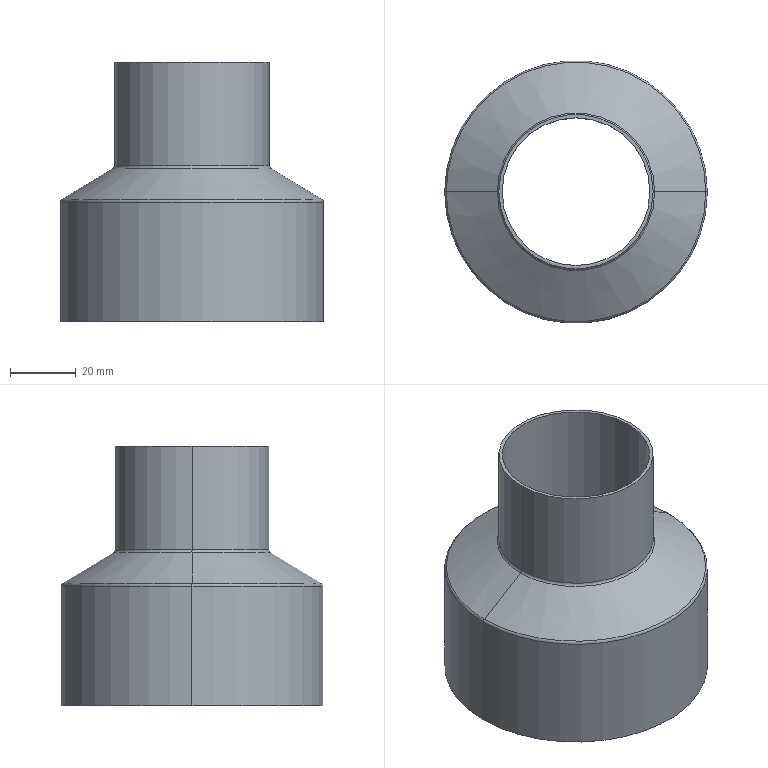Part | SolidWorks | features 3DProfileFeature 2, ICE 2, Blend 1, Fillet 1, Shell 1 | 1 solid | 18 faces | box 80 x 80 x 79 mm | volume 17561 mm3 | cylinder 8 | torus 4 | cone 4 | plane 2 | commonest cylinder face diameters 45 x2 47 x2 78 x2 80 x2
STEP:
#1=CARTESIAN_POINT('',(-23.5,0.,10.563));
#2=VERTEX_POINT('',#1);
#3=CARTESIAN_POINT('',(23.5,0.,10.563));
#4=VERTEX_POINT('',#3);
#5=CARTESIAN_POINT('',(0.,0.,10.563));
#6=DIRECTION('',(0.,0.,1.));
#7=DIRECTION('',(1.,0.,0.));
#8=AXIS2_PLACEMENT_3D('',#5,#6,#7);
#9=CIRCLE('',#8,23.5);
#10=EDGE_CURVE('',#2,#4,#9,.T.);
#11=ORIENTED_EDGE('',*,*,#10,.F.);
#12=CARTESIAN_POINT('',(-23.982,0.,9.708));
#13=VERTEX_POINT('',#12);
#14=CARTESIAN_POINT('',(-24.5,0.,10.563));
#15=DIRECTION('',(0.,1.,0.));
#16=DIRECTION('',(-1.,0.,0.));
#17=AXIS2_PLACEMENT_3D('',#14,#15,#16);
#18=CIRCLE('',#17,1.);
#19=EDGE_CURVE('',#2,#13,#18,.T.);
#20=ORIENTED_EDGE('',*,*,#19,.T.);
#21=CARTESIAN_POINT('',(23.982,0.,9.708));
#22=VERTEX_POINT('',#21);
#23=CARTESIAN_POINT('',(0.,0.,9.708));
#24=DIRECTION('',(0.,0.,-1.));
#25=DIRECTION('',(1.,0.,0.));
#26=AXIS2_PLACEMENT_3D('',#23,#24,#25);
#27=CIRCLE('',#26,23.982);
#28=EDGE_CURVE('',#22,#13,#27,.T.);
#29=ORIENTED_EDGE('',*,*,#28,.F.);
#30=CARTESIAN_POINT('',(24.5,0.,10.563));
#31=DIRECTION('',(0.,-1.,0.));
#32=DIRECTION('',(0.,0.,-1.));
#33=AXIS2_PLACEMENT_3D('',#30,#31,#32);
#34=CIRCLE('',#33,1.);
#35=EDGE_CURVE('',#4,#22,#34,.T.);
#36=ORIENTED_EDGE('',*,*,#35,.F.);
#37=EDGE_LOOP('',(#11,#20,#29,#36));
#38=FACE_OUTER_BOUND('',#37,.T.);
#39=CARTESIAN_POINT('',(0.,0.,10.563));
#40=DIRECTION('',(0.,0.,1.));
#41=DIRECTION('',(1.,0.,0.));
#42=AXIS2_PLACEMENT_3D('',#39,#40,#41);
#43=TOROIDAL_SURFACE('',#42,24.5,1.);
#44=ADVANCED_FACE('',(#38),#43,.F.);
#45=CARTESIAN_POINT('',(-40.,0.,-0.5633));
#46=VERTEX_POINT('',#45);
#47=CARTESIAN_POINT('',(40.,0.,-0.5633));
#48=VERTEX_POINT('',#47);
#49=CARTESIAN_POINT('',(0.,0.,-0.5633));
#50=DIRECTION('',(0.,0.,-1.));
#51=DIRECTION('',(1.,0.,0.));
#52=AXIS2_PLACEMENT_3D('',#49,#50,#51);
#53=CIRCLE('',#52,40.);
#54=EDGE_CURVE('',#46,#48,#53,.T.);
#55=ORIENTED_EDGE('',*,*,#54,.F.);
#56=CARTESIAN_POINT('',(-39.518,0.,0.2919));
#57=VERTEX_POINT('',#56);
#58=CARTESIAN_POINT('',(-39.,0.,-0.5633));
#59=DIRECTION('',(0.,1.,0.));
#60=DIRECTION('',(-1.,0.,0.));
#61=AXIS2_PLACEMENT_3D('',#58,#59,#60);
#62=CIRCLE('',#61,1.);
#63=EDGE_CURVE('',#46,#57,#62,.T.);
#64=ORIENTED_EDGE('',*,*,#63,.T.);
#65=CARTESIAN_POINT('',(39.518,0.,0.2919));
#66=VERTEX_POINT('',#65);
#67=CARTESIAN_POINT('',(0.,0.,0.2919));
#68=DIRECTION('',(0.,0.,1.));
#69=DIRECTION('',(-1.,0.,0.));
#70=AXIS2_PLACEMENT_3D('',#67,#68,#69);
#71=CIRCLE('',#70,39.518);
#72=EDGE_CURVE('',#66,#57,#71,.T.);
#73=ORIENTED_EDGE('',*,*,#72,.F.);
#74=CARTESIAN_POINT('',(39.,0.,-0.5633));
#75=DIRECTION('',(0.,-1.,0.));
#76=DIRECTION('',(0.,0.,-1.));
#77=AXIS2_PLACEMENT_3D('',#74,#75,#76);
#78=CIRCLE('',#77,1.);
#79=EDGE_CURVE('',#48,#66,#78,.T.);
#80=ORIENTED_EDGE('',*,*,#79,.F.);
#81=EDGE_LOOP('',(#55,#64,#73,#80));
#82=FACE_OUTER_BOUND('',#81,.T.);
#83=CARTESIAN_POINT('',(0.,0.,-0.5633));
#84=DIRECTION('',(0.,0.,1.));
#85=DIRECTION('',(1.,0.,0.));
#86=AXIS2_PLACEMENT_3D('',#83,#84,#85);
#87=TOROIDAL_SURFACE('',#86,39.,1.);
#88=ADVANCED_FACE('',(#82),#87,.T.);
#89=CARTESIAN_POINT('',(-22.5,0.,42.));
#90=VERTEX_POINT('',#89);
#91=CARTESIAN_POINT('',(22.5,0.,42.));
#92=VERTEX_POINT('',#91);
#93=CARTESIAN_POINT('',(0.,0.,42.));
#94=DIRECTION('',(0.,0.,1.));
#95=DIRECTION('',(1.,0.,0.));
#96=AXIS2_PLACEMENT_3D('',#93,#94,#95);
#97=CIRCLE('',#96,22.5);
#98=EDGE_CURVE('',#90,#92,#97,.T.);
#99=ORIENTED_EDGE('',*,*,#98,.T.);
#100=CARTESIAN_POINT('',(22.5,0.,9.437));
#101=VERTEX_POINT('',#100);
#102=CARTESIAN_POINT('',(22.5,0.,42.));
#103=DIRECTION('',(0.,0.,-1.));
#104=VECTOR('',#103,1000.);
#105=LINE('',#102,#104);
#106=EDGE_CURVE('',#92,#101,#105,.T.);
#107=ORIENTED_EDGE('',*,*,#106,.T.);
#108=CARTESIAN_POINT('',(-22.5,0.,9.437));
#109=VERTEX_POINT('',#108);
#110=CARTESIAN_POINT('',(0.,0.,9.437));
#111=DIRECTION('',(0.,0.,1.));
#112=DIRECTION('',(-1.,0.,0.));
#113=AXIS2_PLACEMENT_3D('',#110,#111,#112);
#114=CIRCLE('',#113,22.5);
#115=EDGE_CURVE('',#109,#101,#114,.T.);
#116=ORIENTED_EDGE('',*,*,#115,.F.);
#117=CARTESIAN_POINT('',(-22.5,0.,42.));
#118=DIRECTION('',(0.,0.,-1.));
#119=VECTOR('',#118,1000.);
#120=LINE('',#117,#119);
#121=EDGE_CURVE('',#90,#109,#120,.T.);
#122=ORIENTED_EDGE('',*,*,#121,.F.);
#123=EDGE_LOOP('',(#99,#107,#116,#122));
#124=FACE_OUTER_BOUND('',#123,.T.);
#125=CARTESIAN_POINT('',(0.,0.,42.));
#126=DIRECTION('',(0.,0.,-1.));
#127=DIRECTION('',(-1.,0.,0.));
#128=AXIS2_PLACEMENT_3D('',#125,#126,#127);
#129=CYLINDRICAL_SURFACE('',#128,22.5);
#130=ADVANCED_FACE('',(#124),#129,.F.);
#131=CARTESIAN_POINT('',(39.,0.,-37.));
#132=VERTEX_POINT('',#131);
#133=CARTESIAN_POINT('',(-39.,0.,-37.));
#134=VERTEX_POINT('',#133);
#135=CARTESIAN_POINT('',(0.,0.,-37.));
#136=DIRECTION('',(0.,0.,-1.));
#137=DIRECTION('',(-1.,0.,0.));
#138=AXIS2_PLACEMENT_3D('',#135,#136,#137);
#139=CIRCLE('',#138,39.);
#140=EDGE_CURVE('',#132,#134,#139,.T.);
#141=ORIENTED_EDGE('',*,*,#140,.T.);
#142=CARTESIAN_POINT('',(-39.,0.,-0.5633));
#143=VERTEX_POINT('',#142);
#144=CARTESIAN_POINT('',(-39.,0.,-37.));
#145=DIRECTION('',(0.,0.,1.));
#146=VECTOR('',#145,1000.);
#147=LINE('',#144,#146);
#148=EDGE_CURVE('',#134,#143,#147,.T.);
#149=ORIENTED_EDGE('',*,*,#148,.T.);
#150=CARTESIAN_POINT('',(39.,0.,-0.5633));
#151=VERTEX_POINT('',#150);
#152=CARTESIAN_POINT('',(0.,0.,-0.5633));
#153=DIRECTION('',(0.,0.,-1.));
#154=DIRECTION('',(-1.,0.,0.));
#155=AXIS2_PLACEMENT_3D('',#152,#153,#154);
#156=CIRCLE('',#155,39.);
#157=EDGE_CURVE('',#151,#143,#156,.T.);
#158=ORIENTED_EDGE('',*,*,#157,.F.);
#159=CARTESIAN_POINT('',(39.,0.,-37.));
#160=DIRECTION('',(0.,0.,1.));
#161=VECTOR('',#160,1000.);
#162=LINE('',#159,#161);
#163=EDGE_CURVE('',#132,#151,#162,.T.);
#164=ORIENTED_EDGE('',*,*,#163,.F.);
#165=EDGE_LOOP('',(#141,#149,#158,#164));
#166=FACE_OUTER_BOUND('',#165,.T.);
#167=CARTESIAN_POINT('',(0.,0.,-37.));
#168=DIRECTION('',(0.,0.,1.));
#169=DIRECTION('',(1.,0.,0.));
#170=AXIS2_PLACEMENT_3D('',#167,#168,#169);
#171=CYLINDRICAL_SURFACE('',#170,39.);
#172=ADVANCED_FACE('',(#166),#171,.F.);
#173=ORIENTED_EDGE('',*,*,#115,.T.);
#174=CARTESIAN_POINT('',(22.982,0.,9.145));
#175=DIRECTION('',(0.8552,0.,-0.5183));
#176=VECTOR('',#175,1000.);
#177=LINE('',#174,#176);
#178=EDGE_CURVE('',#101,#151,#177,.T.);
#179=ORIENTED_EDGE('',*,*,#178,.T.);
#180=ORIENTED_EDGE('',*,*,#157,.T.);
#181=CARTESIAN_POINT('',(-22.982,0.,9.145));
#182=DIRECTION('',(-0.8552,0.,-0.5183));
#183=VECTOR('',#182,1000.);
#184=LINE('',#181,#183);
#185=EDGE_CURVE('',#109,#143,#184,.T.);
#186=ORIENTED_EDGE('',*,*,#185,.F.);
#187=EDGE_LOOP('',(#173,#179,#180,#186));
#188=FACE_OUTER_BOUND('',#187,.T.);
#189=CARTESIAN_POINT('',(0.,0.,9.145));
#190=DIRECTION('',(0.,0.,-1.));
#191=DIRECTION('',(-1.,0.,0.));
#192=AXIS2_PLACEMENT_3D('',#189,#190,#191);
#193=CONICAL_SURFACE('',#192,22.982,1.026);
#194=ADVANCED_FACE('',(#188),#193,.F.);
#195=CARTESIAN_POINT('',(23.5,0.,42.));
#196=VERTEX_POINT('',#195);
#197=CARTESIAN_POINT('',(-23.5,0.,42.));
#198=VERTEX_POINT('',#197);
#199=CARTESIAN_POINT('',(0.,0.,42.));
#200=DIRECTION('',(0.,0.,1.));
#201=DIRECTION('',(1.,0.,0.));
#202=AXIS2_PLACEMENT_3D('',#199,#200,#201);
#203=CIRCLE('',#202,23.5);
#204=EDGE_CURVE('',#196,#198,#203,.T.);
#205=ORIENTED_EDGE('',*,*,#204,.F.);
#206=CARTESIAN_POINT('',(23.5,0.,42.));
#207=DIRECTION('',(0.,0.,-1.));
#208=VECTOR('',#207,1000.);
#209=LINE('',#206,#208);
#210=EDGE_CURVE('',#196,#4,#209,.T.);
#211=ORIENTED_EDGE('',*,*,#210,.T.);
#212=CARTESIAN_POINT('',(0.,0.,10.563));
#213=DIRECTION('',(0.,0.,1.));
#214=DIRECTION('',(1.,0.,0.));
#215=AXIS2_PLACEMENT_3D('',#212,#213,#214);
#216=CIRCLE('',#215,23.5);
#217=EDGE_CURVE('',#4,#2,#216,.T.);
#218=ORIENTED_EDGE('',*,*,#217,.T.);
#219=CARTESIAN_POINT('',(-23.5,0.,42.));
#220=DIRECTION('',(0.,0.,-1.));
#221=VECTOR('',#220,1000.);
#222=LINE('',#219,#221);
#223=EDGE_CURVE('',#198,#2,#222,.T.);
#224=ORIENTED_EDGE('',*,*,#223,.F.);
#225=EDGE_LOOP('',(#205,#211,#218,#224));
#226=FACE_OUTER_BOUND('',#225,.T.);
#227=CARTESIAN_POINT('',(0.,0.,42.));
#228=DIRECTION('',(0.,0.,-1.));
#229=DIRECTION('',(-1.,0.,0.));
#230=AXIS2_PLACEMENT_3D('',#227,#228,#229);
#231=CYLINDRICAL_SURFACE('',#230,23.5);
#232=ADVANCED_FACE('',(#226),#231,.T.);
#233=CARTESIAN_POINT('',(-40.,0.,-37.));
#234=VERTEX_POINT('',#233);
#235=CARTESIAN_POINT('',(40.,0.,-37.));
#236=VERTEX_POINT('',#235);
#237=CARTESIAN_POINT('',(0.,0.,-37.));
#238=DIRECTION('',(0.,0.,-1.));
#239=DIRECTION('',(-1.,0.,0.));
#240=AXIS2_PLACEMENT_3D('',#237,#238,#239);
#241=CIRCLE('',#240,40.);
#242=EDGE_CURVE('',#234,#236,#241,.T.);
#243=ORIENTED_EDGE('',*,*,#242,.F.);
#244=CARTESIAN_POINT('',(-40.,0.,-37.));
#245=DIRECTION('',(0.,0.,1.));
#246=VECTOR('',#245,1000.);
#247=LINE('',#244,#246);
#248=EDGE_CURVE('',#234,#46,#247,.T.);
#249=ORIENTED_EDGE('',*,*,#248,.T.);
#250=ORIENTED_EDGE('',*,*,#54,.T.);
#251=CARTESIAN_POINT('',(40.,0.,-37.));
#252=DIRECTION('',(0.,0.,1.));
#253=VECTOR('',#252,1000.);
#254=LINE('',#251,#253);
#255=EDGE_CURVE('',#236,#48,#254,.T.);
#256=ORIENTED_EDGE('',*,*,#255,.F.);
#257=EDGE_LOOP('',(#243,#249,#250,#256));
#258=FACE_OUTER_BOUND('',#257,.T.);
#259=CARTESIAN_POINT('',(0.,0.,-37.));
#260=DIRECTION('',(0.,0.,1.));
#261=DIRECTION('',(1.,0.,0.));
#262=AXIS2_PLACEMENT_3D('',#259,#260,#261);
#263=CYLINDRICAL_SURFACE('',#262,40.);
#264=ADVANCED_FACE('',(#258),#263,.T.);
#265=CARTESIAN_POINT('',(0.,0.,9.708));
#266=DIRECTION('',(0.,0.,-1.));
#267=DIRECTION('',(1.,0.,0.));
#268=AXIS2_PLACEMENT_3D('',#265,#266,#267);
#269=CIRCLE('',#268,23.982);
#270=EDGE_CURVE('',#13,#22,#269,.T.);
#271=ORIENTED_EDGE('',*,*,#270,.T.);
#272=CARTESIAN_POINT('',(23.5,0.,10.));
#273=DIRECTION('',(0.8552,0.,-0.5183));
#274=VECTOR('',#273,1000.);
#275=LINE('',#272,#274);
#276=EDGE_CURVE('',#22,#66,#275,.T.);
#277=ORIENTED_EDGE('',*,*,#276,.T.);
#278=ORIENTED_EDGE('',*,*,#72,.T.);
#279=CARTESIAN_POINT('',(-23.5,0.,10.));
#280=DIRECTION('',(-0.8552,0.,-0.5183));
#281=VECTOR('',#280,1000.);
#282=LINE('',#279,#281);
#283=EDGE_CURVE('',#13,#57,#282,.T.);
#284=ORIENTED_EDGE('',*,*,#283,.F.);
#285=EDGE_LOOP('',(#271,#277,#278,#284));
#286=FACE_OUTER_BOUND('',#285,.T.);
#287=CARTESIAN_POINT('',(0.,0.,10.));
#288=DIRECTION('',(0.,0.,-1.));
#289=DIRECTION('',(-1.,0.,0.));
#290=AXIS2_PLACEMENT_3D('',#287,#288,#289);
#291=CONICAL_SURFACE('',#290,23.5,1.026);
#292=ADVANCED_FACE('',(#286),#291,.T.);
#293=ORIENTED_EDGE('',*,*,#276,.F.);
#294=ORIENTED_EDGE('',*,*,#28,.T.);
#295=ORIENTED_EDGE('',*,*,#283,.T.);
#296=CARTESIAN_POINT('',(0.,0.,0.2919));
#297=DIRECTION('',(0.,0.,1.));
#298=DIRECTION('',(-1.,0.,0.));
#299=AXIS2_PLACEMENT_3D('',#296,#297,#298);
#300=CIRCLE('',#299,39.518);
#301=EDGE_CURVE('',#57,#66,#300,.T.);
#302=ORIENTED_EDGE('',*,*,#301,.T.);
#303=EDGE_LOOP('',(#293,#294,#295,#302));
#304=FACE_OUTER_BOUND('',#303,.T.);
#305=CARTESIAN_POINT('',(0.,0.,10.));
#306=DIRECTION('',(0.,0.,-1.));
#307=DIRECTION('',(-1.,0.,0.));
#308=AXIS2_PLACEMENT_3D('',#305,#306,#307);
#309=CONICAL_SURFACE('',#308,23.5,1.026);
#310=ADVANCED_FACE('',(#304),#309,.T.);
#311=ORIENTED_EDGE('',*,*,#248,.F.);
#312=CARTESIAN_POINT('',(0.,0.,-37.));
#313=DIRECTION('',(0.,0.,-1.));
#314=DIRECTION('',(-1.,0.,0.));
#315=AXIS2_PLACEMENT_3D('',#312,#313,#314);
#316=CIRCLE('',#315,40.);
#317=EDGE_CURVE('',#236,#234,#316,.T.);
#318=ORIENTED_EDGE('',*,*,#317,.F.);
#319=ORIENTED_EDGE('',*,*,#255,.T.);
#320=CARTESIAN_POINT('',(0.,0.,-0.5633));
#321=DIRECTION('',(0.,0.,-1.));
#322=DIRECTION('',(1.,0.,0.));
#323=AXIS2_PLACEMENT_3D('',#320,#321,#322);
#324=CIRCLE('',#323,40.);
#325=EDGE_CURVE('',#48,#46,#324,.T.);
#326=ORIENTED_EDGE('',*,*,#325,.T.);
#327=EDGE_LOOP('',(#311,#318,#319,#326));
#328=FACE_OUTER_BOUND('',#327,.T.);
#329=CARTESIAN_POINT('',(0.,0.,-37.));
#330=DIRECTION('',(0.,0.,1.));
#331=DIRECTION('',(1.,0.,0.));
#332=AXIS2_PLACEMENT_3D('',#329,#330,#331);
#333=CYLINDRICAL_SURFACE('',#332,40.);
#334=ADVANCED_FACE('',(#328),#333,.T.);
#335=ORIENTED_EDGE('',*,*,#140,.F.);
#336=CARTESIAN_POINT('',(0.,0.,-37.));
#337=DIRECTION('',(0.,0.,-1.));
#338=DIRECTION('',(-1.,0.,0.));
#339=AXIS2_PLACEMENT_3D('',#336,#337,#338);
#340=CIRCLE('',#339,39.);
#341=EDGE_CURVE('',#134,#132,#340,.T.);
#342=ORIENTED_EDGE('',*,*,#341,.F.);
#343=EDGE_LOOP('',(#335,#342));
#344=FACE_BOUND('',#343,.T.);
#345=ORIENTED_EDGE('',*,*,#317,.T.);
#346=ORIENTED_EDGE('',*,*,#242,.T.);
#347=EDGE_LOOP('',(#345,#346));
#348=FACE_OUTER_BOUND('',#347,.T.);
#349=CARTESIAN_POINT('',(0.,0.,-37.));
#350=DIRECTION('',(0.,0.,-1.));
#351=DIRECTION('',(-1.,0.,0.));
#352=AXIS2_PLACEMENT_3D('',#349,#350,#351);
#353=PLANE('',#352);
#354=ADVANCED_FACE('',(#344,#348),#353,.T.);
#355=ORIENTED_EDGE('',*,*,#210,.F.);
#356=CARTESIAN_POINT('',(0.,0.,42.));
#357=DIRECTION('',(0.,0.,1.));
#358=DIRECTION('',(1.,0.,0.));
#359=AXIS2_PLACEMENT_3D('',#356,#357,#358);
#360=CIRCLE('',#359,23.5);
#361=EDGE_CURVE('',#198,#196,#360,.T.);
#362=ORIENTED_EDGE('',*,*,#361,.F.);
#363=ORIENTED_EDGE('',*,*,#223,.T.);
#364=ORIENTED_EDGE('',*,*,#10,.T.);
#365=EDGE_LOOP('',(#355,#362,#363,#364));
#366=FACE_OUTER_BOUND('',#365,.T.);
#367=CARTESIAN_POINT('',(0.,0.,42.));
#368=DIRECTION('',(0.,0.,-1.));
#369=DIRECTION('',(-1.,0.,0.));
#370=AXIS2_PLACEMENT_3D('',#367,#368,#369);
#371=CYLINDRICAL_SURFACE('',#370,23.5);
#372=ADVANCED_FACE('',(#366),#371,.T.);
#373=ORIENTED_EDGE('',*,*,#98,.F.);
#374=CARTESIAN_POINT('',(0.,0.,42.));
#375=DIRECTION('',(0.,0.,1.));
#376=DIRECTION('',(1.,0.,0.));
#377=AXIS2_PLACEMENT_3D('',#374,#375,#376);
#378=CIRCLE('',#377,22.5);
#379=EDGE_CURVE('',#92,#90,#378,.T.);
#380=ORIENTED_EDGE('',*,*,#379,.F.);
#381=EDGE_LOOP('',(#373,#380));
#382=FACE_BOUND('',#381,.T.);
#383=ORIENTED_EDGE('',*,*,#361,.T.);
#384=ORIENTED_EDGE('',*,*,#204,.T.);
#385=EDGE_LOOP('',(#383,#384));
#386=FACE_OUTER_BOUND('',#385,.T.);
#387=CARTESIAN_POINT('',(0.,0.,42.));
#388=DIRECTION('',(0.,0.,1.));
#389=DIRECTION('',(1.,0.,0.));
#390=AXIS2_PLACEMENT_3D('',#387,#388,#389);
#391=PLANE('',#390);
#392=ADVANCED_FACE('',(#382,#386),#391,.T.);
#393=ORIENTED_EDGE('',*,*,#178,.F.);
#394=CARTESIAN_POINT('',(0.,0.,9.437));
#395=DIRECTION('',(0.,0.,1.));
#396=DIRECTION('',(-1.,0.,0.));
#397=AXIS2_PLACEMENT_3D('',#394,#395,#396);
#398=CIRCLE('',#397,22.5);
#399=EDGE_CURVE('',#101,#109,#398,.T.);
#400=ORIENTED_EDGE('',*,*,#399,.T.);
#401=ORIENTED_EDGE('',*,*,#185,.T.);
#402=CARTESIAN_POINT('',(0.,0.,-0.5633));
#403=DIRECTION('',(0.,0.,-1.));
#404=DIRECTION('',(-1.,0.,0.));
#405=AXIS2_PLACEMENT_3D('',#402,#403,#404);
#406=CIRCLE('',#405,39.);
#407=EDGE_CURVE('',#143,#151,#406,.T.);
#408=ORIENTED_EDGE('',*,*,#407,.T.);
#409=EDGE_LOOP('',(#393,#400,#401,#408));
#410=FACE_OUTER_BOUND('',#409,.T.);
#411=CARTESIAN_POINT('',(0.,0.,9.145));
#412=DIRECTION('',(0.,0.,-1.));
#413=DIRECTION('',(-1.,0.,0.));
#414=AXIS2_PLACEMENT_3D('',#411,#412,#413);
#415=CONICAL_SURFACE('',#414,22.982,1.026);
#416=ADVANCED_FACE('',(#410),#415,.F.);
#417=ORIENTED_EDGE('',*,*,#148,.F.);
#418=ORIENTED_EDGE('',*,*,#341,.T.);
#419=ORIENTED_EDGE('',*,*,#163,.T.);
#420=ORIENTED_EDGE('',*,*,#407,.F.);
#421=EDGE_LOOP('',(#417,#418,#419,#420));
#422=FACE_OUTER_BOUND('',#421,.T.);
#423=CARTESIAN_POINT('',(0.,0.,-37.));
#424=DIRECTION('',(0.,0.,1.));
#425=DIRECTION('',(1.,0.,0.));
#426=AXIS2_PLACEMENT_3D('',#423,#424,#425);
#427=CYLINDRICAL_SURFACE('',#426,39.);
#428=ADVANCED_FACE('',(#422),#427,.F.);
#429=ORIENTED_EDGE('',*,*,#106,.F.);
#430=ORIENTED_EDGE('',*,*,#379,.T.);
#431=ORIENTED_EDGE('',*,*,#121,.T.);
#432=ORIENTED_EDGE('',*,*,#399,.F.);
#433=EDGE_LOOP('',(#429,#430,#431,#432));
#434=FACE_OUTER_BOUND('',#433,.T.);
#435=CARTESIAN_POINT('',(0.,0.,42.));
#436=DIRECTION('',(0.,0.,-1.));
#437=DIRECTION('',(-1.,0.,0.));
#438=AXIS2_PLACEMENT_3D('',#435,#436,#437);
#439=CYLINDRICAL_SURFACE('',#438,22.5);
#440=ADVANCED_FACE('',(#434),#439,.F.);
#441=ORIENTED_EDGE('',*,*,#63,.F.);
#442=ORIENTED_EDGE('',*,*,#325,.F.);
#443=ORIENTED_EDGE('',*,*,#79,.T.);
#444=ORIENTED_EDGE('',*,*,#301,.F.);
#445=EDGE_LOOP('',(#441,#442,#443,#444));
#446=FACE_OUTER_BOUND('',#445,.T.);
#447=CARTESIAN_POINT('',(0.,0.,-0.5633));
#448=DIRECTION('',(0.,0.,1.));
#449=DIRECTION('',(1.,0.,0.));
#450=AXIS2_PLACEMENT_3D('',#447,#448,#449);
#451=TOROIDAL_SURFACE('',#450,39.,1.);
#452=ADVANCED_FACE('',(#446),#451,.T.);
#453=ORIENTED_EDGE('',*,*,#19,.F.);
#454=ORIENTED_EDGE('',*,*,#217,.F.);
#455=ORIENTED_EDGE('',*,*,#35,.T.);
#456=ORIENTED_EDGE('',*,*,#270,.F.);
#457=EDGE_LOOP('',(#453,#454,#455,#456));
#458=FACE_OUTER_BOUND('',#457,.T.);
#459=CARTESIAN_POINT('',(0.,0.,10.563));
#460=DIRECTION('',(0.,0.,1.));
#461=DIRECTION('',(1.,0.,0.));
#462=AXIS2_PLACEMENT_3D('',#459,#460,#461);
#463=TOROIDAL_SURFACE('',#462,24.5,1.);
#464=ADVANCED_FACE('',(#458),#463,.F.);
#465=CLOSED_SHELL('',(#44,#88,#130,#172,#194,#232,#264,#292,#310,#334,#354,#372,#392,#416,#428,#440,#452,#464));
#466=MANIFOLD_SOLID_BREP('',#465);
#467=CARTESIAN_POINT('',(0.,0.,0.));
#468=DIRECTION('',(0.,0.,1.));
#469=DIRECTION('',(1.,0.,0.));
#470=AXIS2_PLACEMENT_3D('',#467,#468,#469);
#471=(LENGTH_UNIT()NAMED_UNIT(*)SI_UNIT(.MILLI.,.METRE.));
#472=UNCERTAINTY_MEASURE_WITH_UNIT(LENGTH_MEASURE(0.00001),#471,'','');
#473=(NAMED_UNIT(*)PLANE_ANGLE_UNIT()SI_UNIT($,.RADIAN.));
#474=(NAMED_UNIT(*)SI_UNIT($,.STERADIAN.)SOLID_ANGLE_UNIT());
#475=(GEOMETRIC_REPRESENTATION_CONTEXT(3)GLOBAL_UNCERTAINTY_ASSIGNED_CONTEXT((#472))GLOBAL_UNIT_ASSIGNED_CONTEXT((#471,#473,#474))REPRESENTATION_CONTEXT('',''));
#476=ADVANCED_BREP_SHAPE_REPRESENTATION('',(#466,#470),#475);